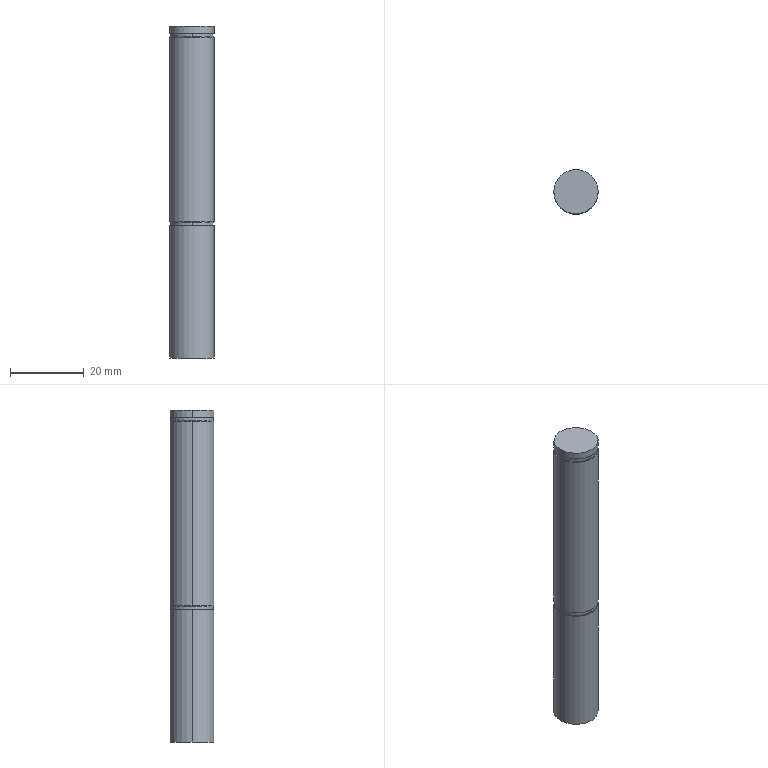Part | SolidWorks | features 3DProfileFeature 3, Extrusion 1, HoleWzd 1, ICE 1, LPattern 1, LibraryFeature 1, RefAxis 1, RevCut 1 | 1 solid | 28 faces | box 12 x 12 x 90 mm | volume 9933 mm3 | cylinder 12 | torus 8 | plane 6 | cone 2 | commonest cylinder face diameters 12 x6 11.5 x4 5 x2
STEP:
#1=CARTESIAN_POINT('',(2.5,0.,11.));
#2=VERTEX_POINT('',#1);
#3=CARTESIAN_POINT('',(-2.5,0.,11.));
#4=VERTEX_POINT('',#3);
#5=CARTESIAN_POINT('',(0.,0.,11.));
#6=DIRECTION('',(0.,0.,-1.));
#7=DIRECTION('',(-1.,0.,0.));
#8=AXIS2_PLACEMENT_3D('',#5,#6,#7);
#9=CIRCLE('',#8,2.5);
#10=EDGE_CURVE('',#2,#4,#9,.T.);
#11=ORIENTED_EDGE('',*,*,#10,.F.);
#12=CARTESIAN_POINT('',(2.5,0.,0.));
#13=VERTEX_POINT('',#12);
#14=CARTESIAN_POINT('',(2.5,0.,0.));
#15=DIRECTION('',(0.,0.,-1.));
#16=VECTOR('',#15,1000.);
#17=LINE('',#14,#16);
#18=EDGE_CURVE('',#2,#13,#17,.T.);
#19=ORIENTED_EDGE('',*,*,#18,.T.);
#20=CARTESIAN_POINT('',(-2.5,0.,0.));
#21=VERTEX_POINT('',#20);
#22=CARTESIAN_POINT('',(0.,0.,0.));
#23=DIRECTION('',(0.,0.,-1.));
#24=DIRECTION('',(-1.,0.,0.));
#25=AXIS2_PLACEMENT_3D('',#22,#23,#24);
#26=CIRCLE('',#25,2.5);
#27=EDGE_CURVE('',#13,#21,#26,.T.);
#28=ORIENTED_EDGE('',*,*,#27,.T.);
#29=CARTESIAN_POINT('',(-2.5,0.,0.));
#30=DIRECTION('',(0.,0.,-1.));
#31=VECTOR('',#30,1000.);
#32=LINE('',#29,#31);
#33=EDGE_CURVE('',#4,#21,#32,.T.);
#34=ORIENTED_EDGE('',*,*,#33,.F.);
#35=EDGE_LOOP('',(#11,#19,#28,#34));
#36=FACE_OUTER_BOUND('',#35,.T.);
#37=CARTESIAN_POINT('',(0.,0.,0.));
#38=DIRECTION('',(0.,0.,-1.));
#39=DIRECTION('',(-1.,0.,0.));
#40=AXIS2_PLACEMENT_3D('',#37,#38,#39);
#41=CYLINDRICAL_SURFACE('',#40,2.5);
#42=ADVANCED_FACE('',(#36),#41,.F.);
#43=CARTESIAN_POINT('',(0.,0.,12.502));
#44=VERTEX_POINT('',#43);
#45=CARTESIAN_POINT('',(-2.5,0.,11.));
#46=DIRECTION('',(-0.8572,0.,-0.515));
#47=VECTOR('',#46,1000.);
#48=LINE('',#45,#47);
#49=EDGE_CURVE('',#44,#4,#48,.T.);
#50=ORIENTED_EDGE('',*,*,#49,.F.);
#51=CARTESIAN_POINT('',(2.5,0.,11.));
#52=DIRECTION('',(0.8572,0.,-0.515));
#53=VECTOR('',#52,1000.);
#54=LINE('',#51,#53);
#55=EDGE_CURVE('',#44,#2,#54,.T.);
#56=ORIENTED_EDGE('',*,*,#55,.T.);
#57=ORIENTED_EDGE('',*,*,#10,.T.);
#58=EDGE_LOOP('',(#50,#56,#57));
#59=FACE_OUTER_BOUND('',#58,.T.);
#60=CARTESIAN_POINT('',(0.,0.,11.));
#61=DIRECTION('',(0.,0.,-1.));
#62=DIRECTION('',(-1.,0.,0.));
#63=AXIS2_PLACEMENT_3D('',#60,#61,#62);
#64=CONICAL_SURFACE('',#63,2.5,1.03);
#65=ADVANCED_FACE('',(#59),#64,.F.);
#66=CARTESIAN_POINT('',(-6.,0.,35.85));
#67=VERTEX_POINT('',#66);
#68=CARTESIAN_POINT('',(6.,0.,35.85));
#69=VERTEX_POINT('',#68);
#70=CARTESIAN_POINT('',(0.,0.,35.85));
#71=DIRECTION('',(0.,0.,-1.));
#72=DIRECTION('',(0.,1.,0.));
#73=AXIS2_PLACEMENT_3D('',#70,#71,#72);
#74=CIRCLE('',#73,6.);
#75=EDGE_CURVE('',#67,#69,#74,.T.);
#76=ORIENTED_EDGE('',*,*,#75,.T.);
#77=CARTESIAN_POINT('',(6.,0.,0.));
#78=VERTEX_POINT('',#77);
#79=CARTESIAN_POINT('',(6.,0.,90.));
#80=DIRECTION('',(0.,0.,-1.));
#81=VECTOR('',#80,1000.);
#82=LINE('',#79,#81);
#83=EDGE_CURVE('',#69,#78,#82,.T.);
#84=ORIENTED_EDGE('',*,*,#83,.T.);
#85=CARTESIAN_POINT('',(-6.,0.,0.));
#86=VERTEX_POINT('',#85);
#87=CARTESIAN_POINT('',(0.,0.,0.));
#88=DIRECTION('',(0.,0.,1.));
#89=DIRECTION('',(1.,0.,0.));
#90=AXIS2_PLACEMENT_3D('',#87,#88,#89);
#91=CIRCLE('',#90,6.);
#92=EDGE_CURVE('',#78,#86,#91,.T.);
#93=ORIENTED_EDGE('',*,*,#92,.T.);
#94=CARTESIAN_POINT('',(-6.,0.,90.));
#95=DIRECTION('',(0.,0.,-1.));
#96=VECTOR('',#95,1000.);
#97=LINE('',#94,#96);
#98=EDGE_CURVE('',#67,#86,#97,.T.);
#99=ORIENTED_EDGE('',*,*,#98,.F.);
#100=EDGE_LOOP('',(#76,#84,#93,#99));
#101=FACE_OUTER_BOUND('',#100,.T.);
#102=CARTESIAN_POINT('',(0.,0.,90.));
#103=DIRECTION('',(0.,0.,-1.));
#104=DIRECTION('',(-1.,0.,0.));
#105=AXIS2_PLACEMENT_3D('',#102,#103,#104);
#106=CYLINDRICAL_SURFACE('',#105,6.);
#107=ADVANCED_FACE('',(#101),#106,.T.);
#108=CARTESIAN_POINT('',(0.,-5.75,36.84));
#109=VERTEX_POINT('',#108);
#110=CARTESIAN_POINT('',(0.,5.75,36.84));
#111=VERTEX_POINT('',#110);
#112=CARTESIAN_POINT('',(0.,0.,36.84));
#113=DIRECTION('',(0.,0.,-1.));
#114=DIRECTION('',(0.,1.,0.));
#115=AXIS2_PLACEMENT_3D('',#112,#113,#114);
#116=CIRCLE('',#115,5.75);
#117=EDGE_CURVE('',#109,#111,#116,.T.);
#118=ORIENTED_EDGE('',*,*,#117,.F.);
#119=CARTESIAN_POINT('',(0.,-5.86,36.95));
#120=VERTEX_POINT('',#119);
#121=CARTESIAN_POINT('',(0.,-5.86,36.84));
#122=DIRECTION('',(1.,0.,0.));
#123=DIRECTION('',(0.,1.,0.));
#124=AXIS2_PLACEMENT_3D('',#121,#122,#123);
#125=CIRCLE('',#124,0.11);
#126=EDGE_CURVE('',#109,#120,#125,.T.);
#127=ORIENTED_EDGE('',*,*,#126,.T.);
#128=CARTESIAN_POINT('',(0.,5.86,36.95));
#129=VERTEX_POINT('',#128);
#130=CARTESIAN_POINT('',(0.,0.,36.95));
#131=DIRECTION('',(0.,0.,-1.));
#132=DIRECTION('',(0.,1.,0.));
#133=AXIS2_PLACEMENT_3D('',#130,#131,#132);
#134=CIRCLE('',#133,5.86);
#135=EDGE_CURVE('',#120,#129,#134,.T.);
#136=ORIENTED_EDGE('',*,*,#135,.T.);
#137=CARTESIAN_POINT('',(0.,5.86,36.84));
#138=DIRECTION('',(-1.,0.,0.));
#139=DIRECTION('',(0.,0.,1.));
#140=AXIS2_PLACEMENT_3D('',#137,#138,#139);
#141=CIRCLE('',#140,0.11);
#142=EDGE_CURVE('',#111,#129,#141,.T.);
#143=ORIENTED_EDGE('',*,*,#142,.F.);
#144=EDGE_LOOP('',(#118,#127,#136,#143));
#145=FACE_OUTER_BOUND('',#144,.T.);
#146=CARTESIAN_POINT('',(0.,0.,36.84));
#147=DIRECTION('',(0.,0.,-1.));
#148=DIRECTION('',(0.,1.,0.));
#149=AXIS2_PLACEMENT_3D('',#146,#147,#148);
#150=TOROIDAL_SURFACE('',#149,5.86,0.11);
#151=ADVANCED_FACE('',(#145),#150,.F.);
#152=CARTESIAN_POINT('',(0.,0.,36.84));
#153=DIRECTION('',(0.,0.,-1.));
#154=DIRECTION('',(0.,1.,0.));
#155=AXIS2_PLACEMENT_3D('',#152,#153,#154);
#156=CIRCLE('',#155,5.75);
#157=EDGE_CURVE('',#111,#109,#156,.T.);
#158=ORIENTED_EDGE('',*,*,#157,.T.);
#159=CARTESIAN_POINT('',(0.,-5.75,35.96));
#160=VERTEX_POINT('',#159);
#161=CARTESIAN_POINT('',(0.,-5.75,-9.58));
#162=DIRECTION('',(0.,0.,-1.));
#163=VECTOR('',#162,1000.);
#164=LINE('',#161,#163);
#165=EDGE_CURVE('',#109,#160,#164,.T.);
#166=ORIENTED_EDGE('',*,*,#165,.T.);
#167=CARTESIAN_POINT('',(0.,5.75,35.96));
#168=VERTEX_POINT('',#167);
#169=CARTESIAN_POINT('',(0.,0.,35.96));
#170=DIRECTION('',(0.,0.,-1.));
#171=DIRECTION('',(0.,1.,0.));
#172=AXIS2_PLACEMENT_3D('',#169,#170,#171);
#173=CIRCLE('',#172,5.75);
#174=EDGE_CURVE('',#168,#160,#173,.T.);
#175=ORIENTED_EDGE('',*,*,#174,.F.);
#176=CARTESIAN_POINT('',(0.,5.75,-9.58));
#177=DIRECTION('',(0.,0.,-1.));
#178=VECTOR('',#177,1000.);
#179=LINE('',#176,#178);
#180=EDGE_CURVE('',#111,#168,#179,.T.);
#181=ORIENTED_EDGE('',*,*,#180,.F.);
#182=EDGE_LOOP('',(#158,#166,#175,#181));
#183=FACE_OUTER_BOUND('',#182,.T.);
#184=CARTESIAN_POINT('',(0.,0.,-9.58));
#185=DIRECTION('',(0.,0.,-1.));
#186=DIRECTION('',(0.,1.,0.));
#187=AXIS2_PLACEMENT_3D('',#184,#185,#186);
#188=CYLINDRICAL_SURFACE('',#187,5.75);
#189=ADVANCED_FACE('',(#183),#188,.T.);
#190=CARTESIAN_POINT('',(0.,-5.86,35.85));
#191=VERTEX_POINT('',#190);
#192=CARTESIAN_POINT('',(0.,5.86,35.85));
#193=VERTEX_POINT('',#192);
#194=CARTESIAN_POINT('',(0.,0.,35.85));
#195=DIRECTION('',(0.,0.,-1.));
#196=DIRECTION('',(0.,1.,0.));
#197=AXIS2_PLACEMENT_3D('',#194,#195,#196);
#198=CIRCLE('',#197,5.86);
#199=EDGE_CURVE('',#191,#193,#198,.T.);
#200=ORIENTED_EDGE('',*,*,#199,.F.);
#201=CARTESIAN_POINT('',(0.,-5.86,35.96));
#202=DIRECTION('',(1.,0.,0.));
#203=DIRECTION('',(0.,1.,0.));
#204=AXIS2_PLACEMENT_3D('',#201,#202,#203);
#205=CIRCLE('',#204,0.11);
#206=EDGE_CURVE('',#191,#160,#205,.T.);
#207=ORIENTED_EDGE('',*,*,#206,.T.);
#208=CARTESIAN_POINT('',(0.,0.,35.96));
#209=DIRECTION('',(0.,0.,-1.));
#210=DIRECTION('',(0.,1.,0.));
#211=AXIS2_PLACEMENT_3D('',#208,#209,#210);
#212=CIRCLE('',#211,5.75);
#213=EDGE_CURVE('',#160,#168,#212,.T.);
#214=ORIENTED_EDGE('',*,*,#213,.T.);
#215=CARTESIAN_POINT('',(0.,5.86,35.96));
#216=DIRECTION('',(-1.,0.,0.));
#217=DIRECTION('',(0.,0.,1.));
#218=AXIS2_PLACEMENT_3D('',#215,#216,#217);
#219=CIRCLE('',#218,0.11);
#220=EDGE_CURVE('',#193,#168,#219,.T.);
#221=ORIENTED_EDGE('',*,*,#220,.F.);
#222=EDGE_LOOP('',(#200,#207,#214,#221));
#223=FACE_OUTER_BOUND('',#222,.T.);
#224=CARTESIAN_POINT('',(0.,0.,35.96));
#225=DIRECTION('',(0.,0.,-1.));
#226=DIRECTION('',(0.,1.,0.));
#227=AXIS2_PLACEMENT_3D('',#224,#225,#226);
#228=TOROIDAL_SURFACE('',#227,5.86,0.11);
#229=ADVANCED_FACE('',(#223),#228,.F.);
#230=CARTESIAN_POINT('',(6.,0.,90.));
#231=VERTEX_POINT('',#230);
#232=CARTESIAN_POINT('',(-6.,0.,90.));
#233=VERTEX_POINT('',#232);
#234=CARTESIAN_POINT('',(0.,0.,90.));
#235=DIRECTION('',(0.,0.,1.));
#236=DIRECTION('',(1.,0.,0.));
#237=AXIS2_PLACEMENT_3D('',#234,#235,#236);
#238=CIRCLE('',#237,6.);
#239=EDGE_CURVE('',#231,#233,#238,.T.);
#240=ORIENTED_EDGE('',*,*,#239,.F.);
#241=CARTESIAN_POINT('',(6.,0.,88.05));
#242=VERTEX_POINT('',#241);
#243=CARTESIAN_POINT('',(6.,0.,90.));
#244=DIRECTION('',(0.,0.,-1.));
#245=VECTOR('',#244,1000.);
#246=LINE('',#243,#245);
#247=EDGE_CURVE('',#231,#242,#246,.T.);
#248=ORIENTED_EDGE('',*,*,#247,.T.);
#249=CARTESIAN_POINT('',(-6.,0.,88.05));
#250=VERTEX_POINT('',#249);
#251=CARTESIAN_POINT('',(0.,0.,88.05));
#252=DIRECTION('',(0.,0.,-1.));
#253=DIRECTION('',(0.,1.,0.));
#254=AXIS2_PLACEMENT_3D('',#251,#252,#253);
#255=CIRCLE('',#254,6.);
#256=EDGE_CURVE('',#250,#242,#255,.T.);
#257=ORIENTED_EDGE('',*,*,#256,.F.);
#258=CARTESIAN_POINT('',(-6.,0.,90.));
#259=DIRECTION('',(0.,0.,-1.));
#260=VECTOR('',#259,1000.);
#261=LINE('',#258,#260);
#262=EDGE_CURVE('',#233,#250,#261,.T.);
#263=ORIENTED_EDGE('',*,*,#262,.F.);
#264=EDGE_LOOP('',(#240,#248,#257,#263));
#265=FACE_OUTER_BOUND('',#264,.T.);
#266=CARTESIAN_POINT('',(0.,0.,90.));
#267=DIRECTION('',(0.,0.,-1.));
#268=DIRECTION('',(-1.,0.,0.));
#269=AXIS2_PLACEMENT_3D('',#266,#267,#268);
#270=CYLINDRICAL_SURFACE('',#269,6.);
#271=ADVANCED_FACE('',(#265),#270,.T.);
#272=CARTESIAN_POINT('',(0.,-5.75,87.94));
#273=VERTEX_POINT('',#272);
#274=CARTESIAN_POINT('',(0.,5.75,87.94));
#275=VERTEX_POINT('',#274);
#276=CARTESIAN_POINT('',(0.,0.,87.94));
#277=DIRECTION('',(0.,0.,-1.));
#278=DIRECTION('',(0.,1.,0.));
#279=AXIS2_PLACEMENT_3D('',#276,#277,#278);
#280=CIRCLE('',#279,5.75);
#281=EDGE_CURVE('',#273,#275,#280,.T.);
#282=ORIENTED_EDGE('',*,*,#281,.F.);
#283=CARTESIAN_POINT('',(0.,-5.86,88.05));
#284=VERTEX_POINT('',#283);
#285=CARTESIAN_POINT('',(0.,-5.86,87.94));
#286=DIRECTION('',(1.,0.,0.));
#287=DIRECTION('',(0.,1.,0.));
#288=AXIS2_PLACEMENT_3D('',#285,#286,#287);
#289=CIRCLE('',#288,0.11);
#290=EDGE_CURVE('',#273,#284,#289,.T.);
#291=ORIENTED_EDGE('',*,*,#290,.T.);
#292=CARTESIAN_POINT('',(0.,5.86,88.05));
#293=VERTEX_POINT('',#292);
#294=CARTESIAN_POINT('',(0.,0.,88.05));
#295=DIRECTION('',(0.,0.,-1.));
#296=DIRECTION('',(0.,1.,0.));
#297=AXIS2_PLACEMENT_3D('',#294,#295,#296);
#298=CIRCLE('',#297,5.86);
#299=EDGE_CURVE('',#284,#293,#298,.T.);
#300=ORIENTED_EDGE('',*,*,#299,.T.);
#301=CARTESIAN_POINT('',(0.,5.86,87.94));
#302=DIRECTION('',(-1.,0.,0.));
#303=DIRECTION('',(0.,0.,1.));
#304=AXIS2_PLACEMENT_3D('',#301,#302,#303);
#305=CIRCLE('',#304,0.11);
#306=EDGE_CURVE('',#275,#293,#305,.T.);
#307=ORIENTED_EDGE('',*,*,#306,.F.);
#308=EDGE_LOOP('',(#282,#291,#300,#307));
#309=FACE_OUTER_BOUND('',#308,.T.);
#310=CARTESIAN_POINT('',(0.,0.,87.94));
#311=DIRECTION('',(0.,0.,-1.));
#312=DIRECTION('',(0.,1.,0.));
#313=AXIS2_PLACEMENT_3D('',#310,#311,#312);
#314=TOROIDAL_SURFACE('',#313,5.86,0.11);
#315=ADVANCED_FACE('',(#309),#314,.F.);
#316=CARTESIAN_POINT('',(0.,0.,87.94));
#317=DIRECTION('',(0.,0.,-1.));
#318=DIRECTION('',(0.,1.,0.));
#319=AXIS2_PLACEMENT_3D('',#316,#317,#318);
#320=CIRCLE('',#319,5.75);
#321=EDGE_CURVE('',#275,#273,#320,.T.);
#322=ORIENTED_EDGE('',*,*,#321,.T.);
#323=CARTESIAN_POINT('',(0.,-5.75,87.06));
#324=VERTEX_POINT('',#323);
#325=CARTESIAN_POINT('',(0.,-5.75,41.52));
#326=DIRECTION('',(0.,0.,-1.));
#327=VECTOR('',#326,1000.);
#328=LINE('',#325,#327);
#329=EDGE_CURVE('',#273,#324,#328,.T.);
#330=ORIENTED_EDGE('',*,*,#329,.T.);
#331=CARTESIAN_POINT('',(0.,5.75,87.06));
#332=VERTEX_POINT('',#331);
#333=CARTESIAN_POINT('',(0.,0.,87.06));
#334=DIRECTION('',(0.,0.,-1.));
#335=DIRECTION('',(0.,1.,0.));
#336=AXIS2_PLACEMENT_3D('',#333,#334,#335);
#337=CIRCLE('',#336,5.75);
#338=EDGE_CURVE('',#332,#324,#337,.T.);
#339=ORIENTED_EDGE('',*,*,#338,.F.);
#340=CARTESIAN_POINT('',(0.,5.75,41.52));
#341=DIRECTION('',(0.,0.,-1.));
#342=VECTOR('',#341,1000.);
#343=LINE('',#340,#342);
#344=EDGE_CURVE('',#275,#332,#343,.T.);
#345=ORIENTED_EDGE('',*,*,#344,.F.);
#346=EDGE_LOOP('',(#322,#330,#339,#345));
#347=FACE_OUTER_BOUND('',#346,.T.);
#348=CARTESIAN_POINT('',(0.,0.,41.52));
#349=DIRECTION('',(0.,0.,-1.));
#350=DIRECTION('',(0.,1.,0.));
#351=AXIS2_PLACEMENT_3D('',#348,#349,#350);
#352=CYLINDRICAL_SURFACE('',#351,5.75);
#353=ADVANCED_FACE('',(#347),#352,.T.);
#354=CARTESIAN_POINT('',(0.,-5.86,86.95));
#355=VERTEX_POINT('',#354);
#356=CARTESIAN_POINT('',(0.,5.86,86.95));
#357=VERTEX_POINT('',#356);
#358=CARTESIAN_POINT('',(0.,0.,86.95));
#359=DIRECTION('',(0.,0.,-1.));
#360=DIRECTION('',(0.,1.,0.));
#361=AXIS2_PLACEMENT_3D('',#358,#359,#360);
#362=CIRCLE('',#361,5.86);
#363=EDGE_CURVE('',#355,#357,#362,.T.);
#364=ORIENTED_EDGE('',*,*,#363,.F.);
#365=CARTESIAN_POINT('',(0.,-5.86,87.06));
#366=DIRECTION('',(1.,0.,0.));
#367=DIRECTION('',(0.,1.,0.));
#368=AXIS2_PLACEMENT_3D('',#365,#366,#367);
#369=CIRCLE('',#368,0.11);
#370=EDGE_CURVE('',#355,#324,#369,.T.);
#371=ORIENTED_EDGE('',*,*,#370,.T.);
#372=CARTESIAN_POINT('',(0.,0.,87.06));
#373=DIRECTION('',(0.,0.,-1.));
#374=DIRECTION('',(0.,1.,0.));
#375=AXIS2_PLACEMENT_3D('',#372,#373,#374);
#376=CIRCLE('',#375,5.75);
#377=EDGE_CURVE('',#324,#332,#376,.T.);
#378=ORIENTED_EDGE('',*,*,#377,.T.);
#379=CARTESIAN_POINT('',(0.,5.86,87.06));
#380=DIRECTION('',(-1.,0.,0.));
#381=DIRECTION('',(0.,0.,1.));
#382=AXIS2_PLACEMENT_3D('',#379,#380,#381);
#383=CIRCLE('',#382,0.11);
#384=EDGE_CURVE('',#357,#332,#383,.T.);
#385=ORIENTED_EDGE('',*,*,#384,.F.);
#386=EDGE_LOOP('',(#364,#371,#378,#385));
#387=FACE_OUTER_BOUND('',#386,.T.);
#388=CARTESIAN_POINT('',(0.,0.,87.06));
#389=DIRECTION('',(0.,0.,-1.));
#390=DIRECTION('',(0.,1.,0.));
#391=AXIS2_PLACEMENT_3D('',#388,#389,#390);
#392=TOROIDAL_SURFACE('',#391,5.86,0.11);
#393=ADVANCED_FACE('',(#387),#392,.F.);
#394=CARTESIAN_POINT('',(-6.,0.,86.95));
#395=VERTEX_POINT('',#394);
#396=CARTESIAN_POINT('',(6.,0.,86.95));
#397=VERTEX_POINT('',#396);
#398=CARTESIAN_POINT('',(0.,0.,86.95));
#399=DIRECTION('',(0.,0.,-1.));
#400=DIRECTION('',(0.,1.,0.));
#401=AXIS2_PLACEMENT_3D('',#398,#399,#400);
#402=CIRCLE('',#401,6.);
#403=EDGE_CURVE('',#395,#397,#402,.T.);
#404=ORIENTED_EDGE('',*,*,#403,.T.);
#405=CARTESIAN_POINT('',(6.,0.,36.95));
#406=VERTEX_POINT('',#405);
#407=CARTESIAN_POINT('',(6.,0.,90.));
#408=DIRECTION('',(0.,0.,-1.));
#409=VECTOR('',#408,1000.);
#410=LINE('',#407,#409);
#411=EDGE_CURVE('',#397,#406,#410,.T.);
#412=ORIENTED_EDGE('',*,*,#411,.T.);
#413=CARTESIAN_POINT('',(-6.,0.,36.95));
#414=VERTEX_POINT('',#413);
#415=CARTESIAN_POINT('',(0.,0.,36.95));
#416=DIRECTION('',(0.,0.,-1.));
#417=DIRECTION('',(0.,1.,0.));
#418=AXIS2_PLACEMENT_3D('',#415,#416,#417);
#419=CIRCLE('',#418,6.);
#420=EDGE_CURVE('',#414,#406,#419,.T.);
#421=ORIENTED_EDGE('',*,*,#420,.F.);
#422=CARTESIAN_POINT('',(-6.,0.,90.));
#423=DIRECTION('',(0.,0.,-1.));
#424=VECTOR('',#423,1000.);
#425=LINE('',#422,#424);
#426=EDGE_CURVE('',#395,#414,#425,.T.);
#427=ORIENTED_EDGE('',*,*,#426,.F.);
#428=EDGE_LOOP('',(#404,#412,#421,#427));
#429=FACE_OUTER_BOUND('',#428,.T.);
#430=CARTESIAN_POINT('',(0.,0.,90.));
#431=DIRECTION('',(0.,0.,-1.));
#432=DIRECTION('',(-1.,0.,0.));
#433=AXIS2_PLACEMENT_3D('',#430,#431,#432);
#434=CYLINDRICAL_SURFACE('',#433,6.);
#435=ADVANCED_FACE('',(#429),#434,.T.);
#436=ORIENTED_EDGE('',*,*,#411,.F.);
#437=CARTESIAN_POINT('',(0.,0.,86.95));
#438=DIRECTION('',(0.,0.,-1.));
#439=DIRECTION('',(0.,1.,0.));
#440=AXIS2_PLACEMENT_3D('',#437,#438,#439);
#441=CIRCLE('',#440,6.);
#442=EDGE_CURVE('',#397,#395,#441,.T.);
#443=ORIENTED_EDGE('',*,*,#442,.T.);
#444=ORIENTED_EDGE('',*,*,#426,.T.);
#445=CARTESIAN_POINT('',(0.,0.,36.95));
#446=DIRECTION('',(0.,0.,-1.));
#447=DIRECTION('',(0.,1.,0.));
#448=AXIS2_PLACEMENT_3D('',#445,#446,#447);
#449=CIRCLE('',#448,6.);
#450=EDGE_CURVE('',#406,#414,#449,.T.);
#451=ORIENTED_EDGE('',*,*,#450,.F.);
#452=EDGE_LOOP('',(#436,#443,#444,#451));
#453=FACE_OUTER_BOUND('',#452,.T.);
#454=CARTESIAN_POINT('',(0.,0.,90.));
#455=DIRECTION('',(0.,0.,-1.));
#456=DIRECTION('',(-1.,0.,0.));
#457=AXIS2_PLACEMENT_3D('',#454,#455,#456);
#458=CYLINDRICAL_SURFACE('',#457,6.);
#459=ADVANCED_FACE('',(#453),#458,.T.);
#460=CARTESIAN_POINT('',(0.,0.,86.95));
#461=DIRECTION('',(0.,0.,-1.));
#462=DIRECTION('',(0.,1.,0.));
#463=AXIS2_PLACEMENT_3D('',#460,#461,#462);
#464=CIRCLE('',#463,5.86);
#465=EDGE_CURVE('',#357,#355,#464,.T.);
#466=ORIENTED_EDGE('',*,*,#465,.T.);
#467=ORIENTED_EDGE('',*,*,#363,.T.);
#468=EDGE_LOOP('',(#466,#467));
#469=FACE_BOUND('',#468,.T.);
#470=ORIENTED_EDGE('',*,*,#403,.F.);
#471=ORIENTED_EDGE('',*,*,#442,.F.);
#472=EDGE_LOOP('',(#470,#471));
#473=FACE_OUTER_BOUND('',#472,.T.);
#474=CARTESIAN_POINT('',(-4.713,-3.713,86.95));
#475=DIRECTION('',(0.,0.,1.));
#476=DIRECTION('',(0.,-1.,0.));
#477=AXIS2_PLACEMENT_3D('',#474,#475,#476);
#478=PLANE('',#477);
#479=ADVANCED_FACE('',(#469,#473),#478,.T.);
#480=ORIENTED_EDGE('',*,*,#370,.F.);
#481=ORIENTED_EDGE('',*,*,#465,.F.);
#482=ORIENTED_EDGE('',*,*,#384,.T.);
#483=ORIENTED_EDGE('',*,*,#338,.T.);
#484=EDGE_LOOP('',(#480,#481,#482,#483));
#485=FACE_OUTER_BOUND('',#484,.T.);
#486=CARTESIAN_POINT('',(0.,0.,87.06));
#487=DIRECTION('',(0.,0.,-1.));
#488=DIRECTION('',(0.,1.,0.));
#489=AXIS2_PLACEMENT_3D('',#486,#487,#488);
#490=TOROIDAL_SURFACE('',#489,5.86,0.11);
#491=ADVANCED_FACE('',(#485),#490,.F.);
#492=ORIENTED_EDGE('',*,*,#329,.F.);
#493=ORIENTED_EDGE('',*,*,#281,.T.);
#494=ORIENTED_EDGE('',*,*,#344,.T.);
#495=ORIENTED_EDGE('',*,*,#377,.F.);
#496=EDGE_LOOP('',(#492,#493,#494,#495));
#497=FACE_OUTER_BOUND('',#496,.T.);
#498=CARTESIAN_POINT('',(0.,0.,41.52));
#499=DIRECTION('',(0.,0.,-1.));
#500=DIRECTION('',(0.,1.,0.));
#501=AXIS2_PLACEMENT_3D('',#498,#499,#500);
#502=CYLINDRICAL_SURFACE('',#501,5.75);
#503=ADVANCED_FACE('',(#497),#502,.T.);
#504=ORIENTED_EDGE('',*,*,#290,.F.);
#505=ORIENTED_EDGE('',*,*,#321,.F.);
#506=ORIENTED_EDGE('',*,*,#306,.T.);
#507=CARTESIAN_POINT('',(0.,0.,88.05));
#508=DIRECTION('',(0.,0.,-1.));
#509=DIRECTION('',(0.,1.,0.));
#510=AXIS2_PLACEMENT_3D('',#507,#508,#509);
#511=CIRCLE('',#510,5.86);
#512=EDGE_CURVE('',#293,#284,#511,.T.);
#513=ORIENTED_EDGE('',*,*,#512,.T.);
#514=EDGE_LOOP('',(#504,#505,#506,#513));
#515=FACE_OUTER_BOUND('',#514,.T.);
#516=CARTESIAN_POINT('',(0.,0.,87.94));
#517=DIRECTION('',(0.,0.,-1.));
#518=DIRECTION('',(0.,1.,0.));
#519=AXIS2_PLACEMENT_3D('',#516,#517,#518);
#520=TOROIDAL_SURFACE('',#519,5.86,0.11);
#521=ADVANCED_FACE('',(#515),#520,.F.);
#522=ORIENTED_EDGE('',*,*,#256,.T.);
#523=CARTESIAN_POINT('',(0.,0.,88.05));
#524=DIRECTION('',(0.,0.,-1.));
#525=DIRECTION('',(0.,1.,0.));
#526=AXIS2_PLACEMENT_3D('',#523,#524,#525);
#527=CIRCLE('',#526,6.);
#528=EDGE_CURVE('',#242,#250,#527,.T.);
#529=ORIENTED_EDGE('',*,*,#528,.T.);
#530=EDGE_LOOP('',(#522,#529));
#531=FACE_OUTER_BOUND('',#530,.T.);
#532=ORIENTED_EDGE('',*,*,#512,.F.);
#533=ORIENTED_EDGE('',*,*,#299,.F.);
#534=EDGE_LOOP('',(#532,#533));
#535=FACE_BOUND('',#534,.T.);
#536=CARTESIAN_POINT('',(-4.603,-3.626,88.05));
#537=DIRECTION('',(0.,0.,-1.));
#538=DIRECTION('',(0.,1.,0.));
#539=AXIS2_PLACEMENT_3D('',#536,#537,#538);
#540=PLANE('',#539);
#541=ADVANCED_FACE('',(#531,#535),#540,.T.);
#542=CARTESIAN_POINT('',(0.,0.,90.));
#543=DIRECTION('',(0.,0.,1.));
#544=DIRECTION('',(1.,0.,0.));
#545=AXIS2_PLACEMENT_3D('',#542,#543,#544);
#546=CIRCLE('',#545,6.);
#547=EDGE_CURVE('',#233,#231,#546,.T.);
#548=ORIENTED_EDGE('',*,*,#547,.T.);
#549=ORIENTED_EDGE('',*,*,#239,.T.);
#550=EDGE_LOOP('',(#548,#549));
#551=FACE_OUTER_BOUND('',#550,.T.);
#552=CARTESIAN_POINT('',(0.,0.,90.));
#553=DIRECTION('',(0.,0.,1.));
#554=DIRECTION('',(1.,0.,0.));
#555=AXIS2_PLACEMENT_3D('',#552,#553,#554);
#556=PLANE('',#555);
#557=ADVANCED_FACE('',(#551),#556,.T.);
#558=ORIENTED_EDGE('',*,*,#247,.F.);
#559=ORIENTED_EDGE('',*,*,#547,.F.);
#560=ORIENTED_EDGE('',*,*,#262,.T.);
#561=ORIENTED_EDGE('',*,*,#528,.F.);
#562=EDGE_LOOP('',(#558,#559,#560,#561));
#563=FACE_OUTER_BOUND('',#562,.T.);
#564=CARTESIAN_POINT('',(0.,0.,90.));
#565=DIRECTION('',(0.,0.,-1.));
#566=DIRECTION('',(-1.,0.,0.));
#567=AXIS2_PLACEMENT_3D('',#564,#565,#566);
#568=CYLINDRICAL_SURFACE('',#567,6.);
#569=ADVANCED_FACE('',(#563),#568,.T.);
#570=CARTESIAN_POINT('',(0.,0.,35.85));
#571=DIRECTION('',(0.,0.,-1.));
#572=DIRECTION('',(0.,1.,0.));
#573=AXIS2_PLACEMENT_3D('',#570,#571,#572);
#574=CIRCLE('',#573,5.86);
#575=EDGE_CURVE('',#193,#191,#574,.T.);
#576=ORIENTED_EDGE('',*,*,#575,.T.);
#577=ORIENTED_EDGE('',*,*,#199,.T.);
#578=EDGE_LOOP('',(#576,#577));
#579=FACE_BOUND('',#578,.T.);
#580=ORIENTED_EDGE('',*,*,#75,.F.);
#581=CARTESIAN_POINT('',(0.,0.,35.85));
#582=DIRECTION('',(0.,0.,-1.));
#583=DIRECTION('',(0.,1.,0.));
#584=AXIS2_PLACEMENT_3D('',#581,#582,#583);
#585=CIRCLE('',#584,6.);
#586=EDGE_CURVE('',#69,#67,#585,.T.);
#587=ORIENTED_EDGE('',*,*,#586,.F.);
#588=EDGE_LOOP('',(#580,#587));
#589=FACE_OUTER_BOUND('',#588,.T.);
#590=CARTESIAN_POINT('',(-4.713,-3.713,35.85));
#591=DIRECTION('',(0.,0.,1.));
#592=DIRECTION('',(0.,-1.,0.));
#593=AXIS2_PLACEMENT_3D('',#590,#591,#592);
#594=PLANE('',#593);
#595=ADVANCED_FACE('',(#579,#589),#594,.T.);
#596=ORIENTED_EDGE('',*,*,#206,.F.);
#597=ORIENTED_EDGE('',*,*,#575,.F.);
#598=ORIENTED_EDGE('',*,*,#220,.T.);
#599=ORIENTED_EDGE('',*,*,#174,.T.);
#600=EDGE_LOOP('',(#596,#597,#598,#599));
#601=FACE_OUTER_BOUND('',#600,.T.);
#602=CARTESIAN_POINT('',(0.,0.,35.96));
#603=DIRECTION('',(0.,0.,-1.));
#604=DIRECTION('',(0.,1.,0.));
#605=AXIS2_PLACEMENT_3D('',#602,#603,#604);
#606=TOROIDAL_SURFACE('',#605,5.86,0.11);
#607=ADVANCED_FACE('',(#601),#606,.F.);
#608=ORIENTED_EDGE('',*,*,#165,.F.);
#609=ORIENTED_EDGE('',*,*,#117,.T.);
#610=ORIENTED_EDGE('',*,*,#180,.T.);
#611=ORIENTED_EDGE('',*,*,#213,.F.);
#612=EDGE_LOOP('',(#608,#609,#610,#611));
#613=FACE_OUTER_BOUND('',#612,.T.);
#614=CARTESIAN_POINT('',(0.,0.,-9.58));
#615=DIRECTION('',(0.,0.,-1.));
#616=DIRECTION('',(0.,1.,0.));
#617=AXIS2_PLACEMENT_3D('',#614,#615,#616);
#618=CYLINDRICAL_SURFACE('',#617,5.75);
#619=ADVANCED_FACE('',(#613),#618,.T.);
#620=ORIENTED_EDGE('',*,*,#126,.F.);
#621=ORIENTED_EDGE('',*,*,#157,.F.);
#622=ORIENTED_EDGE('',*,*,#142,.T.);
#623=CARTESIAN_POINT('',(0.,0.,36.95));
#624=DIRECTION('',(0.,0.,-1.));
#625=DIRECTION('',(0.,1.,0.));
#626=AXIS2_PLACEMENT_3D('',#623,#624,#625);
#627=CIRCLE('',#626,5.86);
#628=EDGE_CURVE('',#129,#120,#627,.T.);
#629=ORIENTED_EDGE('',*,*,#628,.T.);
#630=EDGE_LOOP('',(#620,#621,#622,#629));
#631=FACE_OUTER_BOUND('',#630,.T.);
#632=CARTESIAN_POINT('',(0.,0.,36.84));
#633=DIRECTION('',(0.,0.,-1.));
#634=DIRECTION('',(0.,1.,0.));
#635=AXIS2_PLACEMENT_3D('',#632,#633,#634);
#636=TOROIDAL_SURFACE('',#635,5.86,0.11);
#637=ADVANCED_FACE('',(#631),#636,.F.);
#638=ORIENTED_EDGE('',*,*,#420,.T.);
#639=ORIENTED_EDGE('',*,*,#450,.T.);
#640=EDGE_LOOP('',(#638,#639));
#641=FACE_OUTER_BOUND('',#640,.T.);
#642=ORIENTED_EDGE('',*,*,#628,.F.);
#643=ORIENTED_EDGE('',*,*,#135,.F.);
#644=EDGE_LOOP('',(#642,#643));
#645=FACE_BOUND('',#644,.T.);
#646=CARTESIAN_POINT('',(-4.603,-3.626,36.95));
#647=DIRECTION('',(0.,0.,-1.));
#648=DIRECTION('',(0.,1.,0.));
#649=AXIS2_PLACEMENT_3D('',#646,#647,#648);
#650=PLANE('',#649);
#651=ADVANCED_FACE('',(#641,#645),#650,.T.);
#652=CARTESIAN_POINT('',(0.,0.,0.));
#653=DIRECTION('',(0.,0.,-1.));
#654=DIRECTION('',(-1.,0.,0.));
#655=AXIS2_PLACEMENT_3D('',#652,#653,#654);
#656=CIRCLE('',#655,2.5);
#657=EDGE_CURVE('',#21,#13,#656,.T.);
#658=ORIENTED_EDGE('',*,*,#657,.F.);
#659=ORIENTED_EDGE('',*,*,#27,.F.);
#660=EDGE_LOOP('',(#658,#659));
#661=FACE_BOUND('',#660,.T.);
#662=CARTESIAN_POINT('',(0.,0.,0.));
#663=DIRECTION('',(0.,0.,1.));
#664=DIRECTION('',(1.,0.,0.));
#665=AXIS2_PLACEMENT_3D('',#662,#663,#664);
#666=CIRCLE('',#665,6.);
#667=EDGE_CURVE('',#86,#78,#666,.T.);
#668=ORIENTED_EDGE('',*,*,#667,.F.);
#669=ORIENTED_EDGE('',*,*,#92,.F.);
#670=EDGE_LOOP('',(#668,#669));
#671=FACE_OUTER_BOUND('',#670,.T.);
#672=CARTESIAN_POINT('',(0.,0.,0.));
#673=DIRECTION('',(0.,0.,1.));
#674=DIRECTION('',(1.,0.,0.));
#675=AXIS2_PLACEMENT_3D('',#672,#673,#674);
#676=PLANE('',#675);
#677=ADVANCED_FACE('',(#661,#671),#676,.F.);
#678=ORIENTED_EDGE('',*,*,#83,.F.);
#679=ORIENTED_EDGE('',*,*,#586,.T.);
#680=ORIENTED_EDGE('',*,*,#98,.T.);
#681=ORIENTED_EDGE('',*,*,#667,.T.);
#682=EDGE_LOOP('',(#678,#679,#680,#681));
#683=FACE_OUTER_BOUND('',#682,.T.);
#684=CARTESIAN_POINT('',(0.,0.,90.));
#685=DIRECTION('',(0.,0.,-1.));
#686=DIRECTION('',(-1.,0.,0.));
#687=AXIS2_PLACEMENT_3D('',#684,#685,#686);
#688=CYLINDRICAL_SURFACE('',#687,6.);
#689=ADVANCED_FACE('',(#683),#688,.T.);
#690=ORIENTED_EDGE('',*,*,#55,.F.);
#691=ORIENTED_EDGE('',*,*,#49,.T.);
#692=CARTESIAN_POINT('',(0.,0.,11.));
#693=DIRECTION('',(0.,0.,-1.));
#694=DIRECTION('',(-1.,0.,0.));
#695=AXIS2_PLACEMENT_3D('',#692,#693,#694);
#696=CIRCLE('',#695,2.5);
#697=EDGE_CURVE('',#4,#2,#696,.T.);
#698=ORIENTED_EDGE('',*,*,#697,.T.);
#699=EDGE_LOOP('',(#690,#691,#698));
#700=FACE_OUTER_BOUND('',#699,.T.);
#701=CARTESIAN_POINT('',(0.,0.,11.));
#702=DIRECTION('',(0.,0.,-1.));
#703=DIRECTION('',(-1.,0.,0.));
#704=AXIS2_PLACEMENT_3D('',#701,#702,#703);
#705=CONICAL_SURFACE('',#704,2.5,1.03);
#706=ADVANCED_FACE('',(#700),#705,.F.);
#707=ORIENTED_EDGE('',*,*,#18,.F.);
#708=ORIENTED_EDGE('',*,*,#697,.F.);
#709=ORIENTED_EDGE('',*,*,#33,.T.);
#710=ORIENTED_EDGE('',*,*,#657,.T.);
#711=EDGE_LOOP('',(#707,#708,#709,#710));
#712=FACE_OUTER_BOUND('',#711,.T.);
#713=CARTESIAN_POINT('',(0.,0.,0.));
#714=DIRECTION('',(0.,0.,-1.));
#715=DIRECTION('',(-1.,0.,0.));
#716=AXIS2_PLACEMENT_3D('',#713,#714,#715);
#717=CYLINDRICAL_SURFACE('',#716,2.5);
#718=ADVANCED_FACE('',(#712),#717,.F.);
#719=CLOSED_SHELL('',(#42,#65,#107,#151,#189,#229,#271,#315,#353,#393,#435,#459,#479,#491,#503,#521,#541,#557,#569,#595,#607,#619,#637,#651,#677,#689,#706,#718));
#720=MANIFOLD_SOLID_BREP('',#719);
#721=CARTESIAN_POINT('',(0.,0.,0.));
#722=DIRECTION('',(0.,0.,1.));
#723=DIRECTION('',(1.,0.,0.));
#724=AXIS2_PLACEMENT_3D('',#721,#722,#723);
#725=(LENGTH_UNIT()NAMED_UNIT(*)SI_UNIT(.MILLI.,.METRE.));
#726=UNCERTAINTY_MEASURE_WITH_UNIT(LENGTH_MEASURE(0.00001),#725,'','');
#727=(NAMED_UNIT(*)PLANE_ANGLE_UNIT()SI_UNIT($,.RADIAN.));
#728=(NAMED_UNIT(*)SI_UNIT($,.STERADIAN.)SOLID_ANGLE_UNIT());
#729=(GEOMETRIC_REPRESENTATION_CONTEXT(3)GLOBAL_UNCERTAINTY_ASSIGNED_CONTEXT((#726))GLOBAL_UNIT_ASSIGNED_CONTEXT((#725,#727,#728))REPRESENTATION_CONTEXT('',''));
#730=ADVANCED_BREP_SHAPE_REPRESENTATION('',(#720,#724),#729);